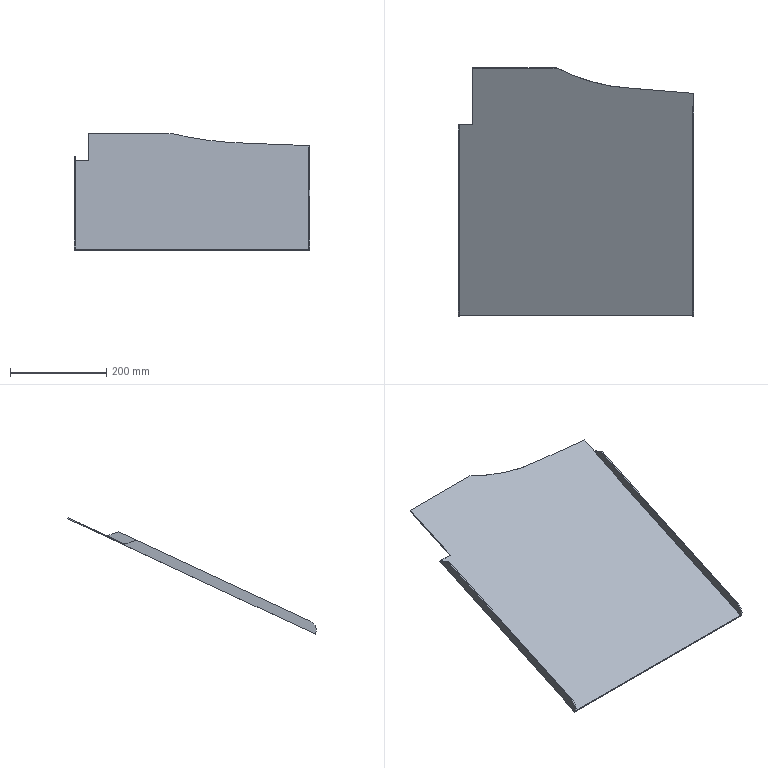Part | NX | features solid 2 | 1 solid | 17 faces | box 490 x 516.322 x 241.704 mm | volume 557231 mm3 | plane 14 | cylinder 2 | spline 1 | commonest cylinder face diameters 40 x2
STEP:
#1=CARTESIAN_POINT('',(-808.,-307.984,-104.35));
#2=VERTEX_POINT('',#1);
#3=CARTESIAN_POINT('',(-808.,-670.326,-273.313));
#4=VERTEX_POINT('',#3);
#5=CARTESIAN_POINT('',(-808.,-303.452,-102.237));
#6=DIRECTION('',(0.,0.9063,0.4226));
#7=VECTOR('',#6,1000.);
#8=LINE('',#5,#7);
#9=EDGE_CURVE('',#2,#4,#8,.F.);
#10=ORIENTED_EDGE('',*,*,#9,.F.);
#11=CARTESIAN_POINT('',(-810.,-307.984,-104.35));
#12=VERTEX_POINT('',#11);
#13=CARTESIAN_POINT('',(-800.,-307.984,-104.35));
#14=DIRECTION('',(1.,0.,0.));
#15=VECTOR('',#14,1000.);
#16=LINE('',#13,#15);
#17=EDGE_CURVE('',#2,#12,#16,.F.);
#18=ORIENTED_EDGE('',*,*,#17,.T.);
#19=CARTESIAN_POINT('',(-810.,-670.326,-273.313));
#20=VERTEX_POINT('',#19);
#21=CARTESIAN_POINT('',(-810.,-2.443,38.126));
#22=DIRECTION('',(0.,0.9063,0.4226));
#23=VECTOR('',#22,1000.);
#24=LINE('',#21,#23);
#25=EDGE_CURVE('',#12,#20,#24,.F.);
#26=ORIENTED_EDGE('',*,*,#25,.T.);
#27=CARTESIAN_POINT('',(-800.,-670.326,-273.313));
#28=DIRECTION('',(1.,0.,0.));
#29=VECTOR('',#28,1000.);
#30=LINE('',#27,#29);
#31=EDGE_CURVE('',#20,#4,#30,.T.);
#32=ORIENTED_EDGE('',*,*,#31,.T.);
#33=EDGE_LOOP('',(#10,#18,#26,#32));
#34=FACE_BOUND('',#33,.T.);
#35=CARTESIAN_POINT('',(-800.,-303.452,-102.237));
#36=DIRECTION('',(0.,0.4226,-0.9063));
#37=DIRECTION('',(0.,-0.9063,-0.4226));
#38=AXIS2_PLACEMENT_3D('',#35,#36,#37);
#39=PLANE('',#38);
#40=ADVANCED_FACE('',(#34),#39,.F.);
#41=CARTESIAN_POINT('',(-808.,-284.063,-113.056));
#42=VERTEX_POINT('',#41);
#43=CARTESIAN_POINT('',(-808.,-680.,-297.684));
#44=VERTEX_POINT('',#43);
#45=CARTESIAN_POINT('',(-808.,-570.845,-246.785));
#46=DIRECTION('',(0.,-0.9063,-0.4226));
#47=VECTOR('',#46,1000.);
#48=LINE('',#45,#47);
#49=EDGE_CURVE('',#42,#44,#48,.T.);
#50=ORIENTED_EDGE('',*,*,#49,.F.);
#51=CARTESIAN_POINT('',(-808.,-307.984,-104.35));
#52=DIRECTION('',(0.,0.9397,-0.342));
#53=VECTOR('',#52,1000.);
#54=LINE('',#51,#53);
#55=EDGE_CURVE('',#42,#2,#54,.F.);
#56=ORIENTED_EDGE('',*,*,#55,.T.);
#57=ORIENTED_EDGE('',*,*,#9,.T.);
#58=CARTESIAN_POINT('',(-808.,-680.,-299.891));
#59=VERTEX_POINT('',#58);
#60=CARTESIAN_POINT('',(-808.,-661.874,-291.439));
#61=DIRECTION('',(-1.,0.,0.));
#62=DIRECTION('',(0.,0.,1.));
#63=AXIS2_PLACEMENT_3D('',#60,#61,#62);
#64=CIRCLE('',#63,20.);
#65=EDGE_CURVE('',#4,#59,#64,.F.);
#66=ORIENTED_EDGE('',*,*,#65,.T.);
#67=CARTESIAN_POINT('',(-808.,-680.,-430.));
#68=DIRECTION('',(0.,0.,1.));
#69=VECTOR('',#68,1000.);
#70=LINE('',#67,#69);
#71=EDGE_CURVE('',#44,#59,#70,.F.);
#72=ORIENTED_EDGE('',*,*,#71,.F.);
#73=EDGE_LOOP('',(#50,#56,#57,#66,#72));
#74=FACE_BOUND('',#73,.T.);
#75=CARTESIAN_POINT('',(-808.,-295.,-120.363));
#76=DIRECTION('',(-1.,0.,0.));
#77=DIRECTION('',(0.,0.,1.));
#78=AXIS2_PLACEMENT_3D('',#75,#76,#77);
#79=PLANE('',#78);
#80=ADVANCED_FACE('',(#74),#79,.F.);
#81=CARTESIAN_POINT('',(-780.,-166.397,-58.187));
#82=VERTEX_POINT('',#81);
#83=CARTESIAN_POINT('',(-780.,-165.552,-60.));
#84=VERTEX_POINT('',#83);
#85=CARTESIAN_POINT('',(-780.,-166.397,-58.187));
#86=DIRECTION('',(0.,0.4226,-0.9063));
#87=VECTOR('',#86,1000.);
#88=LINE('',#85,#87);
#89=EDGE_CURVE('',#82,#84,#88,.T.);
#90=ORIENTED_EDGE('',*,*,#89,.F.);
#91=CARTESIAN_POINT('',(-604.477,-166.397,-58.187));
#92=VERTEX_POINT('',#91);
#93=CARTESIAN_POINT('',(-283.631,-166.397,-58.187));
#94=DIRECTION('',(-1.,0.,0.));
#95=VECTOR('',#94,1000.);
#96=LINE('',#93,#95);
#97=EDGE_CURVE('',#92,#82,#96,.T.);
#98=ORIENTED_EDGE('',*,*,#97,.F.);
#99=CARTESIAN_POINT('',(-606.189,-165.552,-60.));
#100=VERTEX_POINT('',#99);
#101=CARTESIAN_POINT('',(-604.477,-166.397,-58.187));
#102=CARTESIAN_POINT('',(-605.049,-166.116,-58.79));
#103=CARTESIAN_POINT('',(-605.62,-165.834,-59.395));
#104=CARTESIAN_POINT('',(-606.189,-165.552,-60.));
#105=B_SPLINE_CURVE_WITH_KNOTS('',3,(#101,#102,#103,#104),.UNSPECIFIED.,.F.,.F.,(4,4),(0.,0.002633),.UNSPECIFIED.);
#106=EDGE_CURVE('',#92,#100,#105,.T.);
#107=ORIENTED_EDGE('',*,*,#106,.T.);
#108=CARTESIAN_POINT('',(-283.631,-165.552,-60.));
#109=DIRECTION('',(-1.,0.,0.));
#110=VECTOR('',#109,1000.);
#111=LINE('',#108,#110);
#112=EDGE_CURVE('',#100,#84,#111,.T.);
#113=ORIENTED_EDGE('',*,*,#112,.T.);
#114=EDGE_LOOP('',(#90,#98,#107,#113));
#115=FACE_BOUND('',#114,.T.);
#116=CARTESIAN_POINT('',(-283.631,-166.397,-58.187));
#117=DIRECTION('',(0.,-0.9063,-0.4226));
#118=DIRECTION('',(0.,0.4226,-0.9063));
#119=AXIS2_PLACEMENT_3D('',#116,#117,#118);
#120=PLANE('',#119);
#121=ADVANCED_FACE('',(#115),#120,.F.);
#122=CARTESIAN_POINT('',(-780.,-284.063,-113.056));
#123=VERTEX_POINT('',#122);
#124=CARTESIAN_POINT('',(-780.,-570.845,-246.785));
#125=DIRECTION('',(0.,-0.9063,-0.4226));
#126=VECTOR('',#125,1000.);
#127=LINE('',#124,#126);
#128=EDGE_CURVE('',#82,#123,#127,.T.);
#129=ORIENTED_EDGE('',*,*,#128,.F.);
#130=ORIENTED_EDGE('',*,*,#89,.T.);
#131=CARTESIAN_POINT('',(-780.,-283.218,-114.869));
#132=VERTEX_POINT('',#131);
#133=CARTESIAN_POINT('',(-780.,-570.,-248.597));
#134=DIRECTION('',(0.,-0.9063,-0.4226));
#135=VECTOR('',#134,1000.);
#136=LINE('',#133,#135);
#137=EDGE_CURVE('',#84,#132,#136,.T.);
#138=ORIENTED_EDGE('',*,*,#137,.T.);
#139=CARTESIAN_POINT('',(-780.,-284.063,-113.056));
#140=DIRECTION('',(0.,0.4226,-0.9063));
#141=VECTOR('',#140,1000.);
#142=LINE('',#139,#141);
#143=EDGE_CURVE('',#123,#132,#142,.T.);
#144=ORIENTED_EDGE('',*,*,#143,.F.);
#145=EDGE_LOOP('',(#129,#130,#138,#144));
#146=FACE_BOUND('',#145,.T.);
#147=CARTESIAN_POINT('',(-780.,-570.845,-246.785));
#148=DIRECTION('',(1.,0.,0.));
#149=DIRECTION('',(0.,0.,-1.));
#150=AXIS2_PLACEMENT_3D('',#147,#148,#149);
#151=PLANE('',#150);
#152=ADVANCED_FACE('',(#146),#151,.F.);
#153=CARTESIAN_POINT('',(-810.,-284.063,-113.056));
#154=VERTEX_POINT('',#153);
#155=CARTESIAN_POINT('',(-810.,-283.218,-114.869));
#156=VERTEX_POINT('',#155);
#157=CARTESIAN_POINT('',(-810.,-284.063,-113.056));
#158=DIRECTION('',(0.,0.4226,-0.9063));
#159=VECTOR('',#158,1000.);
#160=LINE('',#157,#159);
#161=EDGE_CURVE('',#154,#156,#160,.T.);
#162=ORIENTED_EDGE('',*,*,#161,.F.);
#163=CARTESIAN_POINT('',(-798.,-284.063,-113.056));
#164=DIRECTION('',(1.,0.,0.));
#165=VECTOR('',#164,1000.);
#166=LINE('',#163,#165);
#167=EDGE_CURVE('',#154,#42,#166,.T.);
#168=ORIENTED_EDGE('',*,*,#167,.T.);
#169=CARTESIAN_POINT('',(-800.,-284.063,-113.056));
#170=DIRECTION('',(-1.,0.,0.));
#171=VECTOR('',#170,1000.);
#172=LINE('',#169,#171);
#173=EDGE_CURVE('',#123,#42,#172,.T.);
#174=ORIENTED_EDGE('',*,*,#173,.F.);
#175=ORIENTED_EDGE('',*,*,#143,.T.);
#176=CARTESIAN_POINT('',(-800.,-283.218,-114.869));
#177=DIRECTION('',(-1.,0.,0.));
#178=VECTOR('',#177,1000.);
#179=LINE('',#176,#178);
#180=EDGE_CURVE('',#132,#156,#179,.T.);
#181=ORIENTED_EDGE('',*,*,#180,.T.);
#182=EDGE_LOOP('',(#162,#168,#174,#175,#181));
#183=FACE_BOUND('',#182,.T.);
#184=CARTESIAN_POINT('',(-800.,-284.063,-113.056));
#185=DIRECTION('',(0.,-0.9063,-0.4226));
#186=DIRECTION('',(0.,0.4226,-0.9063));
#187=AXIS2_PLACEMENT_3D('',#184,#185,#186);
#188=PLANE('',#187);
#189=ADVANCED_FACE('',(#183),#188,.F.);
#190=ORIENTED_EDGE('',*,*,#25,.F.);
#191=CARTESIAN_POINT('',(-810.,-307.984,-104.35));
#192=DIRECTION('',(0.,-0.9397,0.342));
#193=VECTOR('',#192,1000.);
#194=LINE('',#191,#193);
#195=EDGE_CURVE('',#12,#154,#194,.F.);
#196=ORIENTED_EDGE('',*,*,#195,.T.);
#197=ORIENTED_EDGE('',*,*,#161,.T.);
#198=CARTESIAN_POINT('',(-810.,-680.,-299.891));
#199=VERTEX_POINT('',#198);
#200=CARTESIAN_POINT('',(-810.,6.009,20.));
#201=DIRECTION('',(0.,-0.9063,-0.4226));
#202=VECTOR('',#201,1000.);
#203=LINE('',#200,#202);
#204=EDGE_CURVE('',#156,#199,#203,.T.);
#205=ORIENTED_EDGE('',*,*,#204,.T.);
#206=CARTESIAN_POINT('',(-810.,-661.874,-291.439));
#207=DIRECTION('',(1.,0.,0.));
#208=DIRECTION('',(0.,0.,-1.));
#209=AXIS2_PLACEMENT_3D('',#206,#207,#208);
#210=CIRCLE('',#209,20.);
#211=EDGE_CURVE('',#199,#20,#210,.F.);
#212=ORIENTED_EDGE('',*,*,#211,.T.);
#213=EDGE_LOOP('',(#190,#196,#197,#205,#212));
#214=FACE_BOUND('',#213,.T.);
#215=CARTESIAN_POINT('',(-810.,5.164,21.813));
#216=DIRECTION('',(1.,0.,0.));
#217=DIRECTION('',(0.,0.,-1.));
#218=AXIS2_PLACEMENT_3D('',#215,#216,#217);
#219=PLANE('',#218);
#220=ADVANCED_FACE('',(#214),#219,.F.);
#221=ORIENTED_EDGE('',*,*,#211,.F.);
#222=CARTESIAN_POINT('',(-800.,-680.,-299.891));
#223=DIRECTION('',(1.,0.,0.));
#224=VECTOR('',#223,1000.);
#225=LINE('',#222,#224);
#226=EDGE_CURVE('',#199,#59,#225,.T.);
#227=ORIENTED_EDGE('',*,*,#226,.T.);
#228=ORIENTED_EDGE('',*,*,#65,.F.);
#229=ORIENTED_EDGE('',*,*,#31,.F.);
#230=EDGE_LOOP('',(#221,#227,#228,#229));
#231=FACE_BOUND('',#230,.T.);
#232=CARTESIAN_POINT('',(-800.,-661.874,-291.439));
#233=DIRECTION('',(-1.,0.,0.));
#234=DIRECTION('',(0.,0.,1.));
#235=AXIS2_PLACEMENT_3D('',#232,#233,#234);
#236=CYLINDRICAL_SURFACE('',#235,20.);
#237=ADVANCED_FACE('',(#231),#236,.T.);
#238=CARTESIAN_POINT('',(-320.,-680.,-299.891));
#239=VERTEX_POINT('',#238);
#240=CARTESIAN_POINT('',(-322.,-680.,-299.891));
#241=VERTEX_POINT('',#240);
#242=CARTESIAN_POINT('',(188.564,-680.,-299.891));
#243=DIRECTION('',(1.,0.,0.));
#244=VECTOR('',#243,1000.);
#245=LINE('',#242,#244);
#246=EDGE_CURVE('',#239,#241,#245,.F.);
#247=ORIENTED_EDGE('',*,*,#246,.T.);
#248=CARTESIAN_POINT('',(188.564,-680.,-299.891));
#249=DIRECTION('',(1.,0.,0.));
#250=VECTOR('',#249,1000.);
#251=LINE('',#248,#250);
#252=EDGE_CURVE('',#241,#59,#251,.F.);
#253=ORIENTED_EDGE('',*,*,#252,.T.);
#254=ORIENTED_EDGE('',*,*,#226,.F.);
#255=ORIENTED_EDGE('',*,*,#204,.F.);
#256=ORIENTED_EDGE('',*,*,#180,.F.);
#257=ORIENTED_EDGE('',*,*,#137,.F.);
#258=ORIENTED_EDGE('',*,*,#112,.F.);
#259=CARTESIAN_POINT('',(-320.,-218.75,-84.807));
#260=VERTEX_POINT('',#259);
#261=CARTESIAN_POINT('',(-320.,-218.75,-84.807));
#262=CARTESIAN_POINT('',(-332.246,-217.754,-84.342));
#263=CARTESIAN_POINT('',(-356.739,-215.761,-83.413));
#264=CARTESIAN_POINT('',(-387.355,-213.269,-82.251));
#265=CARTESIAN_POINT('',(-411.848,-211.277,-81.322));
#266=CARTESIAN_POINT('',(-430.218,-209.78,-80.624));
#267=CARTESIAN_POINT('',(-445.527,-208.539,-80.045));
#268=CARTESIAN_POINT('',(-457.772,-207.533,-79.576));
#269=CARTESIAN_POINT('',(-466.96,-206.815,-79.242));
#270=CARTESIAN_POINT('',(-476.131,-205.957,-78.841));
#271=CARTESIAN_POINT('',(-488.321,-204.401,-78.116));
#272=CARTESIAN_POINT('',(-503.421,-201.823,-76.914));
#273=CARTESIAN_POINT('',(-521.297,-197.753,-75.016));
#274=CARTESIAN_POINT('',(-544.796,-191.122,-71.924));
#275=CARTESIAN_POINT('',(-573.389,-180.849,-67.133));
#276=CARTESIAN_POINT('',(-595.397,-170.904,-62.496));
#277=CARTESIAN_POINT('',(-606.189,-165.552,-60.));
#278=B_SPLINE_CURVE_WITH_KNOTS('',3,(#261,#262,#263,#264,#265,#266,#267,#268,#269,#270,#271,#272,#273,#274,#275,#276,#277),.UNSPECIFIED.,.F.,.F.,(4,1,1,1,1,1,1,1,1,1,1,1,1,1,4),(0.,0.03689,0.07377,0.09222,0.1107,0.1291,0.1383,0.1475,0.1568,0.166,0.1844,0.2029,0.2213,0.2582,0.2951),.UNSPECIFIED.);
#279=EDGE_CURVE('',#260,#100,#278,.T.);
#280=ORIENTED_EDGE('',*,*,#279,.F.);
#281=CARTESIAN_POINT('',(-320.,-570.,-248.597));
#282=DIRECTION('',(0.,-0.9063,-0.4226));
#283=VECTOR('',#282,1000.);
#284=LINE('',#281,#283);
#285=EDGE_CURVE('',#260,#239,#284,.T.);
#286=ORIENTED_EDGE('',*,*,#285,.T.);
#287=EDGE_LOOP('',(#247,#253,#254,#255,#256,#257,#258,#280,#286));
#288=FACE_BOUND('',#287,.T.);
#289=CARTESIAN_POINT('',(-800.,-570.,-248.597));
#290=DIRECTION('',(0.,-0.4226,0.9063));
#291=DIRECTION('',(0.,-0.9063,-0.4226));
#292=AXIS2_PLACEMENT_3D('',#289,#290,#291);
#293=PLANE('',#292);
#294=ADVANCED_FACE('',(#288),#293,.F.);
#295=CARTESIAN_POINT('',(-320.,-218.75,-82.6));
#296=VERTEX_POINT('',#295);
#297=CARTESIAN_POINT('',(-320.,-218.75,-82.6));
#298=CARTESIAN_POINT('',(-332.165,-217.76,-82.139));
#299=CARTESIAN_POINT('',(-356.496,-215.78,-81.215));
#300=CARTESIAN_POINT('',(-386.909,-213.306,-80.061));
#301=CARTESIAN_POINT('',(-411.24,-211.325,-79.138));
#302=CARTESIAN_POINT('',(-429.488,-209.844,-78.447));
#303=CARTESIAN_POINT('',(-447.735,-208.345,-77.748));
#304=CARTESIAN_POINT('',(-462.947,-207.151,-77.191));
#305=CARTESIAN_POINT('',(-475.101,-206.073,-76.688));
#306=CARTESIAN_POINT('',(-487.212,-204.564,-75.985));
#307=CARTESIAN_POINT('',(-502.229,-202.057,-74.816));
#308=CARTESIAN_POINT('',(-520.,-198.079,-72.961));
#309=CARTESIAN_POINT('',(-543.377,-191.578,-69.93));
#310=CARTESIAN_POINT('',(-571.824,-181.474,-65.218));
#311=CARTESIAN_POINT('',(-593.732,-171.675,-60.649));
#312=CARTESIAN_POINT('',(-604.477,-166.397,-58.187));
#313=B_SPLINE_CURVE_WITH_KNOTS('',3,(#297,#298,#299,#300,#301,#302,#303,#304,#305,#306,#307,#308,#309,#310,#311,#312),.UNSPECIFIED.,.F.,.F.,(4,1,1,1,1,1,1,1,1,1,1,1,1,4),(0.,0.03664,0.07329,0.09161,0.1099,0.1282,0.1466,0.1557,0.1649,0.1832,0.2015,0.2199,0.2565,0.2931),.UNSPECIFIED.);
#314=EDGE_CURVE('',#296,#92,#313,.T.);
#315=ORIENTED_EDGE('',*,*,#314,.F.);
#316=CARTESIAN_POINT('',(-320.,-218.75,-83.704));
#317=DIRECTION('',(0.,0.,-1.));
#318=VECTOR('',#317,1000.);
#319=LINE('',#316,#318);
#320=EDGE_CURVE('',#296,#260,#319,.T.);
#321=ORIENTED_EDGE('',*,*,#320,.T.);
#322=ORIENTED_EDGE('',*,*,#279,.T.);
#323=ORIENTED_EDGE('',*,*,#106,.F.);
#324=EDGE_LOOP('',(#315,#321,#322,#323));
#325=FACE_BOUND('',#324,.T.);
#326=CARTESIAN_POINT('',(-607.76,-164.769,-58.028));
#327=CARTESIAN_POINT('',(-607.76,-164.769,-84.967));
#328=CARTESIAN_POINT('',(-596.795,-170.255,-58.028));
#329=CARTESIAN_POINT('',(-596.795,-170.255,-84.967));
#330=CARTESIAN_POINT('',(-574.473,-180.42,-58.028));
#331=CARTESIAN_POINT('',(-574.473,-180.42,-84.967));
#332=CARTESIAN_POINT('',(-545.662,-190.84,-58.028));
#333=CARTESIAN_POINT('',(-545.662,-190.84,-84.967));
#334=CARTESIAN_POINT('',(-522.151,-197.534,-58.028));
#335=CARTESIAN_POINT('',(-522.151,-197.534,-84.967));
#336=CARTESIAN_POINT('',(-504.3,-201.645,-58.028));
#337=CARTESIAN_POINT('',(-504.3,-201.645,-84.967));
#338=CARTESIAN_POINT('',(-489.279,-204.255,-58.028));
#339=CARTESIAN_POINT('',(-489.279,-204.255,-84.967));
#340=CARTESIAN_POINT('',(-477.175,-205.834,-58.028));
#341=CARTESIAN_POINT('',(-477.175,-205.834,-84.967));
#342=CARTESIAN_POINT('',(-468.126,-206.727,-58.028));
#343=CARTESIAN_POINT('',(-468.126,-206.727,-84.967));
#344=CARTESIAN_POINT('',(-458.845,-207.444,-58.028));
#345=CARTESIAN_POINT('',(-458.845,-207.444,-84.967));
#346=CARTESIAN_POINT('',(-446.511,-208.46,-58.028));
#347=CARTESIAN_POINT('',(-446.511,-208.46,-84.967));
#348=CARTESIAN_POINT('',(-431.079,-209.71,-58.028));
#349=CARTESIAN_POINT('',(-431.079,-209.71,-84.967));
#350=CARTESIAN_POINT('',(-412.567,-211.218,-58.028));
#351=CARTESIAN_POINT('',(-412.567,-211.218,-84.967));
#352=CARTESIAN_POINT('',(-387.882,-213.226,-58.028));
#353=CARTESIAN_POINT('',(-387.882,-213.226,-84.967));
#354=CARTESIAN_POINT('',(-357.027,-215.737,-58.028));
#355=CARTESIAN_POINT('',(-357.027,-215.737,-84.967));
#356=CARTESIAN_POINT('',(-332.342,-217.746,-58.028));
#357=CARTESIAN_POINT('',(-332.342,-217.746,-84.967));
#358=CARTESIAN_POINT('',(-320.,-218.75,-58.028));
#359=CARTESIAN_POINT('',(-320.,-218.75,-84.967));
#360=B_SPLINE_SURFACE_WITH_KNOTS('',3,1,((#326,#327),(#328,#329),(#330,#331),(#332,#333),(#334,#335),(#336,#337),(#338,#339),(#340,#341),(#342,#343),(#344,#345),(#346,#347),(#348,#349),(#350,#351),(#352,#353),(#354,#355),(#356,#357),(#358,#359)),.SURF_OF_LINEAR_EXTRUSION.,.F.,.F.,.F.,(4,1,1,1,1,1,1,1,1,1,1,1,1,1,4),(2,2),(0.04006,0.2781,0.5162,0.6353,0.7543,0.8734,0.9329,0.9924,1.052,1.111,1.23,1.35,1.469,1.707,1.945),(0.,1.),.UNSPECIFIED.);
#361=ADVANCED_FACE('',(#325),#360,.T.);
#362=CARTESIAN_POINT('',(-322.,-246.626,-95.599));
#363=VERTEX_POINT('',#362);
#364=CARTESIAN_POINT('',(-322.,-680.,-297.684));
#365=VERTEX_POINT('',#364);
#366=CARTESIAN_POINT('',(-322.,-570.845,-246.785));
#367=DIRECTION('',(0.,-0.9063,-0.4226));
#368=VECTOR('',#367,1000.);
#369=LINE('',#366,#368);
#370=EDGE_CURVE('',#363,#365,#369,.T.);
#371=ORIENTED_EDGE('',*,*,#370,.F.);
#372=CARTESIAN_POINT('',(-320.,-246.626,-95.599));
#373=VERTEX_POINT('',#372);
#374=CARTESIAN_POINT('',(-800.,-246.626,-95.599));
#375=DIRECTION('',(1.,0.,0.));
#376=VECTOR('',#375,1000.);
#377=LINE('',#374,#376);
#378=EDGE_CURVE('',#373,#363,#377,.F.);
#379=ORIENTED_EDGE('',*,*,#378,.F.);
#380=CARTESIAN_POINT('',(-320.,-570.845,-246.785));
#381=DIRECTION('',(0.,-0.9063,-0.4226));
#382=VECTOR('',#381,1000.);
#383=LINE('',#380,#382);
#384=EDGE_CURVE('',#296,#373,#383,.T.);
#385=ORIENTED_EDGE('',*,*,#384,.F.);
#386=ORIENTED_EDGE('',*,*,#314,.T.);
#387=ORIENTED_EDGE('',*,*,#97,.T.);
#388=ORIENTED_EDGE('',*,*,#128,.T.);
#389=ORIENTED_EDGE('',*,*,#173,.T.);
#390=ORIENTED_EDGE('',*,*,#49,.T.);
#391=CARTESIAN_POINT('',(188.564,-680.,-297.684));
#392=DIRECTION('',(1.,0.,0.));
#393=VECTOR('',#392,1000.);
#394=LINE('',#391,#393);
#395=EDGE_CURVE('',#365,#44,#394,.F.);
#396=ORIENTED_EDGE('',*,*,#395,.F.);
#397=EDGE_LOOP('',(#371,#379,#385,#386,#387,#388,#389,#390,#396));
#398=FACE_BOUND('',#397,.T.);
#399=CARTESIAN_POINT('',(-800.,-570.845,-246.785));
#400=DIRECTION('',(0.,-0.4226,0.9063));
#401=DIRECTION('',(0.,-0.9063,-0.4226));
#402=AXIS2_PLACEMENT_3D('',#399,#400,#401);
#403=PLANE('',#402);
#404=ADVANCED_FACE('',(#398),#403,.T.);
#405=CARTESIAN_POINT('',(-322.,-680.,-430.));
#406=DIRECTION('',(0.,0.,1.));
#407=VECTOR('',#406,1000.);
#408=LINE('',#405,#407);
#409=EDGE_CURVE('',#365,#241,#408,.F.);
#410=ORIENTED_EDGE('',*,*,#409,.F.);
#411=ORIENTED_EDGE('',*,*,#395,.T.);
#412=ORIENTED_EDGE('',*,*,#71,.T.);
#413=ORIENTED_EDGE('',*,*,#252,.F.);
#414=EDGE_LOOP('',(#410,#411,#412,#413));
#415=FACE_BOUND('',#414,.T.);
#416=CARTESIAN_POINT('',(188.564,-680.,-430.));
#417=DIRECTION('',(0.,1.,0.));
#418=DIRECTION('',(-1.,0.,0.));
#419=AXIS2_PLACEMENT_3D('',#416,#417,#418);
#420=PLANE('',#419);
#421=ADVANCED_FACE('',(#415),#420,.F.);
#422=ORIENTED_EDGE('',*,*,#384,.T.);
#423=CARTESIAN_POINT('',(-320.,-270.547,-86.893));
#424=VERTEX_POINT('',#423);
#425=CARTESIAN_POINT('',(-320.,-270.547,-86.893));
#426=DIRECTION('',(0.,0.9397,-0.342));
#427=VECTOR('',#426,1000.);
#428=LINE('',#425,#427);
#429=EDGE_CURVE('',#373,#424,#428,.F.);
#430=ORIENTED_EDGE('',*,*,#429,.T.);
#431=CARTESIAN_POINT('',(-320.,-670.326,-273.313));
#432=VERTEX_POINT('',#431);
#433=CARTESIAN_POINT('',(-320.,-252.421,-78.44));
#434=DIRECTION('',(0.,-0.9063,-0.4226));
#435=VECTOR('',#434,1000.);
#436=LINE('',#433,#435);
#437=EDGE_CURVE('',#424,#432,#436,.T.);
#438=ORIENTED_EDGE('',*,*,#437,.T.);
#439=CARTESIAN_POINT('',(-320.,-661.874,-291.439));
#440=DIRECTION('',(-1.,0.,0.));
#441=DIRECTION('',(0.,0.,1.));
#442=AXIS2_PLACEMENT_3D('',#439,#440,#441);
#443=CIRCLE('',#442,20.);
#444=EDGE_CURVE('',#432,#239,#443,.F.);
#445=ORIENTED_EDGE('',*,*,#444,.T.);
#446=ORIENTED_EDGE('',*,*,#285,.F.);
#447=ORIENTED_EDGE('',*,*,#320,.F.);
#448=EDGE_LOOP('',(#422,#430,#438,#445,#446,#447));
#449=FACE_BOUND('',#448,.T.);
#450=CARTESIAN_POINT('',(-320.,-570.,-55.));
#451=DIRECTION('',(-1.,0.,0.));
#452=DIRECTION('',(0.,0.,1.));
#453=AXIS2_PLACEMENT_3D('',#450,#451,#452);
#454=PLANE('',#453);
#455=ADVANCED_FACE('',(#449),#454,.F.);
#456=CARTESIAN_POINT('',(-322.,-270.547,-86.893));
#457=VERTEX_POINT('',#456);
#458=CARTESIAN_POINT('',(-322.,-670.326,-273.313));
#459=VERTEX_POINT('',#458);
#460=CARTESIAN_POINT('',(-322.,-252.421,-78.44));
#461=DIRECTION('',(0.,-0.9063,-0.4226));
#462=VECTOR('',#461,1000.);
#463=LINE('',#460,#462);
#464=EDGE_CURVE('',#457,#459,#463,.T.);
#465=ORIENTED_EDGE('',*,*,#464,.T.);
#466=CARTESIAN_POINT('',(-320.,-670.326,-273.313));
#467=DIRECTION('',(1.,0.,0.));
#468=VECTOR('',#467,1000.);
#469=LINE('',#466,#468);
#470=EDGE_CURVE('',#459,#432,#469,.T.);
#471=ORIENTED_EDGE('',*,*,#470,.T.);
#472=ORIENTED_EDGE('',*,*,#437,.F.);
#473=CARTESIAN_POINT('',(-320.,-270.547,-86.893));
#474=DIRECTION('',(-1.,0.,0.));
#475=VECTOR('',#474,1000.);
#476=LINE('',#473,#475);
#477=EDGE_CURVE('',#424,#457,#476,.T.);
#478=ORIENTED_EDGE('',*,*,#477,.T.);
#479=EDGE_LOOP('',(#465,#471,#472,#478));
#480=FACE_BOUND('',#479,.T.);
#481=CARTESIAN_POINT('',(-320.,-252.421,-78.44));
#482=DIRECTION('',(0.,0.4226,-0.9063));
#483=DIRECTION('',(0.,-0.9063,-0.4226));
#484=AXIS2_PLACEMENT_3D('',#481,#482,#483);
#485=PLANE('',#484);
#486=ADVANCED_FACE('',(#480),#485,.F.);
#487=CARTESIAN_POINT('',(-322.,-243.969,-96.566));
#488=DIRECTION('',(0.,-0.9397,0.342));
#489=VECTOR('',#488,1000.);
#490=LINE('',#487,#489);
#491=EDGE_CURVE('',#457,#363,#490,.F.);
#492=ORIENTED_EDGE('',*,*,#491,.T.);
#493=ORIENTED_EDGE('',*,*,#370,.T.);
#494=ORIENTED_EDGE('',*,*,#409,.T.);
#495=CARTESIAN_POINT('',(-322.,-661.874,-291.439));
#496=DIRECTION('',(-1.,0.,0.));
#497=DIRECTION('',(0.,0.,1.));
#498=AXIS2_PLACEMENT_3D('',#495,#496,#497);
#499=CIRCLE('',#498,20.);
#500=EDGE_CURVE('',#241,#459,#499,.T.);
#501=ORIENTED_EDGE('',*,*,#500,.T.);
#502=ORIENTED_EDGE('',*,*,#464,.F.);
#503=EDGE_LOOP('',(#492,#493,#494,#501,#502));
#504=FACE_BOUND('',#503,.T.);
#505=CARTESIAN_POINT('',(-322.,-243.969,-96.566));
#506=DIRECTION('',(-1.,0.,0.));
#507=DIRECTION('',(0.,0.,1.));
#508=AXIS2_PLACEMENT_3D('',#505,#506,#507);
#509=PLANE('',#508);
#510=ADVANCED_FACE('',(#504),#509,.T.);
#511=ORIENTED_EDGE('',*,*,#429,.F.);
#512=ORIENTED_EDGE('',*,*,#378,.T.);
#513=ORIENTED_EDGE('',*,*,#491,.F.);
#514=ORIENTED_EDGE('',*,*,#477,.F.);
#515=EDGE_LOOP('',(#511,#512,#513,#514));
#516=FACE_BOUND('',#515,.T.);
#517=CARTESIAN_POINT('',(-320.,-270.547,-86.893));
#518=DIRECTION('',(0.,-0.342,-0.9397));
#519=DIRECTION('',(0.,0.9397,-0.342));
#520=AXIS2_PLACEMENT_3D('',#517,#518,#519);
#521=PLANE('',#520);
#522=ADVANCED_FACE('',(#516),#521,.F.);
#523=ORIENTED_EDGE('',*,*,#444,.F.);
#524=ORIENTED_EDGE('',*,*,#470,.F.);
#525=ORIENTED_EDGE('',*,*,#500,.F.);
#526=ORIENTED_EDGE('',*,*,#246,.F.);
#527=EDGE_LOOP('',(#523,#524,#525,#526));
#528=FACE_BOUND('',#527,.T.);
#529=CARTESIAN_POINT('',(-320.,-661.874,-291.439));
#530=DIRECTION('',(1.,0.,0.));
#531=DIRECTION('',(0.,0.,-1.));
#532=AXIS2_PLACEMENT_3D('',#529,#530,#531);
#533=CYLINDRICAL_SURFACE('',#532,20.);
#534=ADVANCED_FACE('',(#528),#533,.T.);
#535=ORIENTED_EDGE('',*,*,#55,.F.);
#536=ORIENTED_EDGE('',*,*,#167,.F.);
#537=ORIENTED_EDGE('',*,*,#195,.F.);
#538=ORIENTED_EDGE('',*,*,#17,.F.);
#539=EDGE_LOOP('',(#535,#536,#537,#538));
#540=FACE_BOUND('',#539,.T.);
#541=CARTESIAN_POINT('',(-800.,-307.984,-104.35));
#542=DIRECTION('',(0.,-0.342,-0.9397));
#543=DIRECTION('',(0.,0.9397,-0.342));
#544=AXIS2_PLACEMENT_3D('',#541,#542,#543);
#545=PLANE('',#544);
#546=ADVANCED_FACE('',(#540),#545,.F.);
#547=CLOSED_SHELL('',(#40,#80,#121,#152,#189,#220,#237,#294,#361,#404,#421,#455,#486,#510,#522,#534,#546));
#548=MANIFOLD_SOLID_BREP('',#547);
#549=(LENGTH_UNIT()NAMED_UNIT(*)SI_UNIT(.MILLI.,.METRE.));
#550=UNCERTAINTY_MEASURE_WITH_UNIT(LENGTH_MEASURE(0.0508),#549,'','');
#551=(NAMED_UNIT(*)PLANE_ANGLE_UNIT()SI_UNIT($,.RADIAN.));
#552=(NAMED_UNIT(*)SI_UNIT($,.STERADIAN.)SOLID_ANGLE_UNIT());
#553=(GEOMETRIC_REPRESENTATION_CONTEXT(3)GLOBAL_UNCERTAINTY_ASSIGNED_CONTEXT((#550))GLOBAL_UNIT_ASSIGNED_CONTEXT((#549,#551,#552))REPRESENTATION_CONTEXT('',''));
#554=ADVANCED_BREP_SHAPE_REPRESENTATION('',(#548),#553);